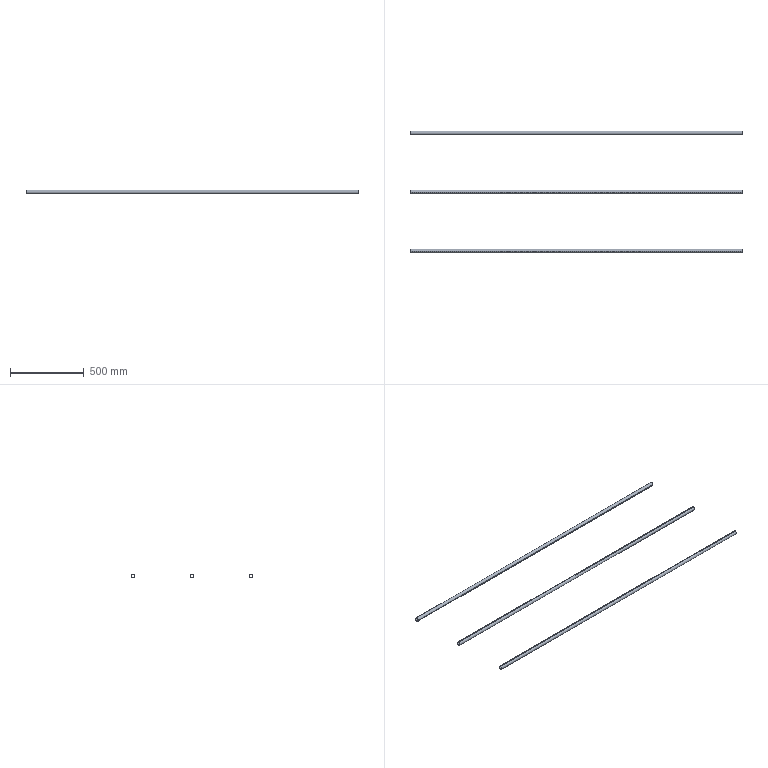Part | STEP file | 粉仓护栏栏杆6_Default<As Machined> | 3 solids | 18 faces | box 2250 x 825 x 25 mm | volume 747503 mm3 | cylinder 12 | plane 6 | commonest cylinder face diameters 22 x6 25 x6
STEP:
#1=CARTESIAN_POINT('',(0.,0.,0.));
#2=DIRECTION('',(0.,0.,1.));
#3=DIRECTION('',(1.,0.,0.));
#4=AXIS2_PLACEMENT_3D('',#1,#2,#3);
#5=CARTESIAN_POINT('',(-2250.,0.,12.5));
#6=VERTEX_POINT('',#5);
#7=CARTESIAN_POINT('',(-2250.,0.,-12.5));
#8=VERTEX_POINT('',#7);
#9=CARTESIAN_POINT('',(-2250.,0.,0.));
#10=DIRECTION('',(-1.,0.,0.));
#11=DIRECTION('',(0.,-1.,0.));
#12=AXIS2_PLACEMENT_3D('',#9,#10,#11);
#13=CIRCLE('',#12,12.5);
#14=CARTESIAN_POINT('',(-2250.,0.,0.));
#15=DIRECTION('',(1.,0.,0.));
#16=DIRECTION('',(0.,0.,-1.));
#17=AXIS2_PLACEMENT_3D('',#14,#15,#16);
#18=CYLINDRICAL_SURFACE('',#17,12.5);
#19=CARTESIAN_POINT('',(4.712,0.));
#20=DIRECTION('',(-1.,0.));
#21=VECTOR('',#20,1.);
#22=LINE('',#19,#21);
#23=(GEOMETRIC_REPRESENTATION_CONTEXT(2)PARAMETRIC_REPRESENTATION_CONTEXT()REPRESENTATION_CONTEXT('',''));
#24=DEFINITIONAL_REPRESENTATION('',(#22),#23);
#25=PCURVE('',#18,#24);
#26=CARTESIAN_POINT('',(-2250.,0.,0.));
#27=DIRECTION('',(-1.,0.,0.));
#28=DIRECTION('',(0.,-1.,0.));
#29=AXIS2_PLACEMENT_3D('',#26,#27,#28);
#30=PLANE('',#29);
#31=CARTESIAN_POINT('',(0.,0.));
#32=DIRECTION('',(1.,0.));
#33=AXIS2_PLACEMENT_2D('',#31,#32);
#34=CIRCLE('',#33,12.5);
#35=(GEOMETRIC_REPRESENTATION_CONTEXT(2)PARAMETRIC_REPRESENTATION_CONTEXT()REPRESENTATION_CONTEXT('',''));
#36=DEFINITIONAL_REPRESENTATION('',(#34),#35);
#37=PCURVE('',#30,#36);
#38=SURFACE_CURVE('',#13,(#25,#37),.PCURVE_S1.);
#39=EDGE_CURVE('',#6,#8,#38,.T.);
#40=ORIENTED_EDGE('',*,*,#39,.F.);
#41=CARTESIAN_POINT('',(0.,0.,12.5));
#42=VERTEX_POINT('',#41);
#43=CARTESIAN_POINT('',(-2250.,0.,12.5));
#44=DIRECTION('',(1.,0.,0.));
#45=VECTOR('',#44,1.);
#46=LINE('',#43,#45);
#47=CARTESIAN_POINT('',(3.142,0.));
#48=DIRECTION('',(0.,1.));
#49=VECTOR('',#48,1.);
#50=LINE('',#47,#49);
#51=(GEOMETRIC_REPRESENTATION_CONTEXT(2)PARAMETRIC_REPRESENTATION_CONTEXT()REPRESENTATION_CONTEXT('',''));
#52=DEFINITIONAL_REPRESENTATION('',(#50),#51);
#53=PCURVE('',#18,#52);
#54=CARTESIAN_POINT('',(-2250.,0.,0.));
#55=DIRECTION('',(1.,0.,0.));
#56=DIRECTION('',(0.,0.,-1.));
#57=AXIS2_PLACEMENT_3D('',#54,#55,#56);
#58=CYLINDRICAL_SURFACE('',#57,12.5);
#59=CARTESIAN_POINT('',(3.142,0.));
#60=DIRECTION('',(0.,1.));
#61=VECTOR('',#60,1.);
#62=LINE('',#59,#61);
#63=(GEOMETRIC_REPRESENTATION_CONTEXT(2)PARAMETRIC_REPRESENTATION_CONTEXT()REPRESENTATION_CONTEXT('',''));
#64=DEFINITIONAL_REPRESENTATION('',(#62),#63);
#65=PCURVE('',#58,#64);
#66=SURFACE_CURVE('',#46,(#53,#65),.PCURVE_S1.);
#67=EDGE_CURVE('',#6,#42,#66,.T.);
#68=ORIENTED_EDGE('',*,*,#67,.T.);
#69=CARTESIAN_POINT('',(0.,0.,-12.5));
#70=VERTEX_POINT('',#69);
#71=CARTESIAN_POINT('',(0.,0.,0.));
#72=DIRECTION('',(-1.,0.,0.));
#73=DIRECTION('',(0.,-1.,0.));
#74=AXIS2_PLACEMENT_3D('',#71,#72,#73);
#75=CIRCLE('',#74,12.5);
#76=CARTESIAN_POINT('',(4.712,2250.));
#77=DIRECTION('',(-1.,0.));
#78=VECTOR('',#77,1.);
#79=LINE('',#76,#78);
#80=(GEOMETRIC_REPRESENTATION_CONTEXT(2)PARAMETRIC_REPRESENTATION_CONTEXT()REPRESENTATION_CONTEXT('',''));
#81=DEFINITIONAL_REPRESENTATION('',(#79),#80);
#82=PCURVE('',#18,#81);
#83=CARTESIAN_POINT('',(0.,0.,0.));
#84=DIRECTION('',(-1.,0.,0.));
#85=DIRECTION('',(0.,-1.,0.));
#86=AXIS2_PLACEMENT_3D('',#83,#84,#85);
#87=PLANE('',#86);
#88=CARTESIAN_POINT('',(0.,0.));
#89=DIRECTION('',(1.,0.));
#90=AXIS2_PLACEMENT_2D('',#88,#89);
#91=CIRCLE('',#90,12.5);
#92=(GEOMETRIC_REPRESENTATION_CONTEXT(2)PARAMETRIC_REPRESENTATION_CONTEXT()REPRESENTATION_CONTEXT('',''));
#93=DEFINITIONAL_REPRESENTATION('',(#91),#92);
#94=PCURVE('',#87,#93);
#95=SURFACE_CURVE('',#75,(#82,#94),.PCURVE_S1.);
#96=EDGE_CURVE('',#42,#70,#95,.T.);
#97=ORIENTED_EDGE('',*,*,#96,.T.);
#98=CARTESIAN_POINT('',(-2250.,0.,-12.5));
#99=DIRECTION('',(1.,0.,0.));
#100=VECTOR('',#99,1.);
#101=LINE('',#98,#100);
#102=CARTESIAN_POINT('',(0.,0.));
#103=DIRECTION('',(0.,1.));
#104=VECTOR('',#103,1.);
#105=LINE('',#102,#104);
#106=(GEOMETRIC_REPRESENTATION_CONTEXT(2)PARAMETRIC_REPRESENTATION_CONTEXT()REPRESENTATION_CONTEXT('',''));
#107=DEFINITIONAL_REPRESENTATION('',(#105),#106);
#108=PCURVE('',#18,#107);
#109=CARTESIAN_POINT('',(6.283,0.));
#110=DIRECTION('',(0.,1.));
#111=VECTOR('',#110,1.);
#112=LINE('',#109,#111);
#113=(GEOMETRIC_REPRESENTATION_CONTEXT(2)PARAMETRIC_REPRESENTATION_CONTEXT()REPRESENTATION_CONTEXT('',''));
#114=DEFINITIONAL_REPRESENTATION('',(#112),#113);
#115=PCURVE('',#58,#114);
#116=SURFACE_CURVE('',#101,(#108,#115),.PCURVE_S1.);
#117=EDGE_CURVE('',#8,#70,#116,.T.);
#118=ORIENTED_EDGE('',*,*,#117,.F.);
#119=EDGE_LOOP('',(#40,#68,#97,#118));
#120=FACE_BOUND('',#119,.T.);
#121=ADVANCED_FACE('',(#120),#18,.T.);
#122=CARTESIAN_POINT('',(-2250.,0.,-11.));
#123=VERTEX_POINT('',#122);
#124=CARTESIAN_POINT('',(0.,0.,-11.));
#125=VERTEX_POINT('',#124);
#126=CARTESIAN_POINT('',(-2250.,0.,-11.));
#127=DIRECTION('',(1.,0.,0.));
#128=VECTOR('',#127,1.);
#129=LINE('',#126,#128);
#130=CARTESIAN_POINT('',(-2250.,0.,0.));
#131=DIRECTION('',(1.,0.,0.));
#132=DIRECTION('',(0.,0.,-1.));
#133=AXIS2_PLACEMENT_3D('',#130,#131,#132);
#134=CYLINDRICAL_SURFACE('',#133,11.);
#135=CARTESIAN_POINT('',(6.283,0.));
#136=DIRECTION('',(0.,1.));
#137=VECTOR('',#136,1.);
#138=LINE('',#135,#137);
#139=(GEOMETRIC_REPRESENTATION_CONTEXT(2)PARAMETRIC_REPRESENTATION_CONTEXT()REPRESENTATION_CONTEXT('',''));
#140=DEFINITIONAL_REPRESENTATION('',(#138),#139);
#141=PCURVE('',#134,#140);
#142=CARTESIAN_POINT('',(-2250.,0.,0.));
#143=DIRECTION('',(1.,0.,0.));
#144=DIRECTION('',(0.,0.,-1.));
#145=AXIS2_PLACEMENT_3D('',#142,#143,#144);
#146=CYLINDRICAL_SURFACE('',#145,11.);
#147=CARTESIAN_POINT('',(0.,0.));
#148=DIRECTION('',(0.,1.));
#149=VECTOR('',#148,1.);
#150=LINE('',#147,#149);
#151=(GEOMETRIC_REPRESENTATION_CONTEXT(2)PARAMETRIC_REPRESENTATION_CONTEXT()REPRESENTATION_CONTEXT('',''));
#152=DEFINITIONAL_REPRESENTATION('',(#150),#151);
#153=PCURVE('',#146,#152);
#154=SURFACE_CURVE('',#129,(#141,#153),.PCURVE_S1.);
#155=EDGE_CURVE('',#123,#125,#154,.T.);
#156=ORIENTED_EDGE('',*,*,#155,.T.);
#157=CARTESIAN_POINT('',(0.,0.,11.));
#158=VERTEX_POINT('',#157);
#159=CARTESIAN_POINT('',(0.,0.,0.));
#160=DIRECTION('',(-1.,0.,0.));
#161=DIRECTION('',(0.,-1.,0.));
#162=AXIS2_PLACEMENT_3D('',#159,#160,#161);
#163=CIRCLE('',#162,11.);
#164=CARTESIAN_POINT('',(10.996,2250.));
#165=DIRECTION('',(-1.,0.));
#166=VECTOR('',#165,1.);
#167=LINE('',#164,#166);
#168=(GEOMETRIC_REPRESENTATION_CONTEXT(2)PARAMETRIC_REPRESENTATION_CONTEXT()REPRESENTATION_CONTEXT('',''));
#169=DEFINITIONAL_REPRESENTATION('',(#167),#168);
#170=PCURVE('',#134,#169);
#171=CARTESIAN_POINT('',(0.,0.));
#172=DIRECTION('',(1.,0.));
#173=AXIS2_PLACEMENT_2D('',#171,#172);
#174=CIRCLE('',#173,11.);
#175=(GEOMETRIC_REPRESENTATION_CONTEXT(2)PARAMETRIC_REPRESENTATION_CONTEXT()REPRESENTATION_CONTEXT('',''));
#176=DEFINITIONAL_REPRESENTATION('',(#174),#175);
#177=PCURVE('',#87,#176);
#178=SURFACE_CURVE('',#163,(#170,#177),.PCURVE_S1.);
#179=EDGE_CURVE('',#125,#158,#178,.T.);
#180=ORIENTED_EDGE('',*,*,#179,.T.);
#181=CARTESIAN_POINT('',(-2250.,0.,11.));
#182=VERTEX_POINT('',#181);
#183=CARTESIAN_POINT('',(-2250.,0.,11.));
#184=DIRECTION('',(1.,0.,0.));
#185=VECTOR('',#184,1.);
#186=LINE('',#183,#185);
#187=CARTESIAN_POINT('',(3.142,0.));
#188=DIRECTION('',(0.,1.));
#189=VECTOR('',#188,1.);
#190=LINE('',#187,#189);
#191=(GEOMETRIC_REPRESENTATION_CONTEXT(2)PARAMETRIC_REPRESENTATION_CONTEXT()REPRESENTATION_CONTEXT('',''));
#192=DEFINITIONAL_REPRESENTATION('',(#190),#191);
#193=PCURVE('',#134,#192);
#194=CARTESIAN_POINT('',(3.142,0.));
#195=DIRECTION('',(0.,1.));
#196=VECTOR('',#195,1.);
#197=LINE('',#194,#196);
#198=(GEOMETRIC_REPRESENTATION_CONTEXT(2)PARAMETRIC_REPRESENTATION_CONTEXT()REPRESENTATION_CONTEXT('',''));
#199=DEFINITIONAL_REPRESENTATION('',(#197),#198);
#200=PCURVE('',#146,#199);
#201=SURFACE_CURVE('',#186,(#193,#200),.PCURVE_S1.);
#202=EDGE_CURVE('',#182,#158,#201,.T.);
#203=ORIENTED_EDGE('',*,*,#202,.F.);
#204=CARTESIAN_POINT('',(-2250.,0.,0.));
#205=DIRECTION('',(-1.,0.,0.));
#206=DIRECTION('',(0.,-1.,0.));
#207=AXIS2_PLACEMENT_3D('',#204,#205,#206);
#208=CIRCLE('',#207,11.);
#209=CARTESIAN_POINT('',(10.996,0.));
#210=DIRECTION('',(-1.,0.));
#211=VECTOR('',#210,1.);
#212=LINE('',#209,#211);
#213=(GEOMETRIC_REPRESENTATION_CONTEXT(2)PARAMETRIC_REPRESENTATION_CONTEXT()REPRESENTATION_CONTEXT('',''));
#214=DEFINITIONAL_REPRESENTATION('',(#212),#213);
#215=PCURVE('',#134,#214);
#216=CARTESIAN_POINT('',(0.,0.));
#217=DIRECTION('',(1.,0.));
#218=AXIS2_PLACEMENT_2D('',#216,#217);
#219=CIRCLE('',#218,11.);
#220=(GEOMETRIC_REPRESENTATION_CONTEXT(2)PARAMETRIC_REPRESENTATION_CONTEXT()REPRESENTATION_CONTEXT('',''));
#221=DEFINITIONAL_REPRESENTATION('',(#219),#220);
#222=PCURVE('',#30,#221);
#223=SURFACE_CURVE('',#208,(#215,#222),.PCURVE_S1.);
#224=EDGE_CURVE('',#123,#182,#223,.T.);
#225=ORIENTED_EDGE('',*,*,#224,.F.);
#226=EDGE_LOOP('',(#156,#180,#203,#225));
#227=FACE_BOUND('',#226,.F.);
#228=ADVANCED_FACE('',(#227),#134,.F.);
#229=CARTESIAN_POINT('',(0.,0.,0.));
#230=DIRECTION('',(-1.,0.,0.));
#231=DIRECTION('',(0.,-1.,0.));
#232=AXIS2_PLACEMENT_3D('',#229,#230,#231);
#233=CIRCLE('',#232,11.);
#234=CARTESIAN_POINT('',(4.712,2250.));
#235=DIRECTION('',(-1.,0.));
#236=VECTOR('',#235,1.);
#237=LINE('',#234,#236);
#238=(GEOMETRIC_REPRESENTATION_CONTEXT(2)PARAMETRIC_REPRESENTATION_CONTEXT()REPRESENTATION_CONTEXT('',''));
#239=DEFINITIONAL_REPRESENTATION('',(#237),#238);
#240=PCURVE('',#146,#239);
#241=CARTESIAN_POINT('',(0.,0.));
#242=DIRECTION('',(1.,0.));
#243=AXIS2_PLACEMENT_2D('',#241,#242);
#244=CIRCLE('',#243,11.);
#245=(GEOMETRIC_REPRESENTATION_CONTEXT(2)PARAMETRIC_REPRESENTATION_CONTEXT()REPRESENTATION_CONTEXT('',''));
#246=DEFINITIONAL_REPRESENTATION('',(#244),#245);
#247=PCURVE('',#87,#246);
#248=SURFACE_CURVE('',#233,(#240,#247),.PCURVE_S1.);
#249=EDGE_CURVE('',#158,#125,#248,.T.);
#250=ORIENTED_EDGE('',*,*,#249,.T.);
#251=ORIENTED_EDGE('',*,*,#155,.F.);
#252=CARTESIAN_POINT('',(-2250.,0.,0.));
#253=DIRECTION('',(-1.,0.,0.));
#254=DIRECTION('',(0.,-1.,0.));
#255=AXIS2_PLACEMENT_3D('',#252,#253,#254);
#256=CIRCLE('',#255,11.);
#257=CARTESIAN_POINT('',(4.712,0.));
#258=DIRECTION('',(-1.,0.));
#259=VECTOR('',#258,1.);
#260=LINE('',#257,#259);
#261=(GEOMETRIC_REPRESENTATION_CONTEXT(2)PARAMETRIC_REPRESENTATION_CONTEXT()REPRESENTATION_CONTEXT('',''));
#262=DEFINITIONAL_REPRESENTATION('',(#260),#261);
#263=PCURVE('',#146,#262);
#264=CARTESIAN_POINT('',(0.,0.));
#265=DIRECTION('',(1.,0.));
#266=AXIS2_PLACEMENT_2D('',#264,#265);
#267=CIRCLE('',#266,11.);
#268=(GEOMETRIC_REPRESENTATION_CONTEXT(2)PARAMETRIC_REPRESENTATION_CONTEXT()REPRESENTATION_CONTEXT('',''));
#269=DEFINITIONAL_REPRESENTATION('',(#267),#268);
#270=PCURVE('',#30,#269);
#271=SURFACE_CURVE('',#256,(#263,#270),.PCURVE_S1.);
#272=EDGE_CURVE('',#182,#123,#271,.T.);
#273=ORIENTED_EDGE('',*,*,#272,.F.);
#274=ORIENTED_EDGE('',*,*,#202,.T.);
#275=EDGE_LOOP('',(#250,#251,#273,#274));
#276=FACE_BOUND('',#275,.F.);
#277=ADVANCED_FACE('',(#276),#146,.F.);
#278=ORIENTED_EDGE('',*,*,#67,.F.);
#279=CARTESIAN_POINT('',(-2250.,0.,0.));
#280=DIRECTION('',(-1.,0.,0.));
#281=DIRECTION('',(0.,-1.,0.));
#282=AXIS2_PLACEMENT_3D('',#279,#280,#281);
#283=CIRCLE('',#282,12.5);
#284=CARTESIAN_POINT('',(10.996,0.));
#285=DIRECTION('',(-1.,0.));
#286=VECTOR('',#285,1.);
#287=LINE('',#284,#286);
#288=(GEOMETRIC_REPRESENTATION_CONTEXT(2)PARAMETRIC_REPRESENTATION_CONTEXT()REPRESENTATION_CONTEXT('',''));
#289=DEFINITIONAL_REPRESENTATION('',(#287),#288);
#290=PCURVE('',#58,#289);
#291=CARTESIAN_POINT('',(0.,0.));
#292=DIRECTION('',(1.,0.));
#293=AXIS2_PLACEMENT_2D('',#291,#292);
#294=CIRCLE('',#293,12.5);
#295=(GEOMETRIC_REPRESENTATION_CONTEXT(2)PARAMETRIC_REPRESENTATION_CONTEXT()REPRESENTATION_CONTEXT('',''));
#296=DEFINITIONAL_REPRESENTATION('',(#294),#295);
#297=PCURVE('',#30,#296);
#298=SURFACE_CURVE('',#283,(#290,#297),.PCURVE_S1.);
#299=EDGE_CURVE('',#8,#6,#298,.T.);
#300=ORIENTED_EDGE('',*,*,#299,.F.);
#301=ORIENTED_EDGE('',*,*,#117,.T.);
#302=CARTESIAN_POINT('',(0.,0.,0.));
#303=DIRECTION('',(-1.,0.,0.));
#304=DIRECTION('',(0.,-1.,0.));
#305=AXIS2_PLACEMENT_3D('',#302,#303,#304);
#306=CIRCLE('',#305,12.5);
#307=CARTESIAN_POINT('',(10.996,2250.));
#308=DIRECTION('',(-1.,0.));
#309=VECTOR('',#308,1.);
#310=LINE('',#307,#309);
#311=(GEOMETRIC_REPRESENTATION_CONTEXT(2)PARAMETRIC_REPRESENTATION_CONTEXT()REPRESENTATION_CONTEXT('',''));
#312=DEFINITIONAL_REPRESENTATION('',(#310),#311);
#313=PCURVE('',#58,#312);
#314=CARTESIAN_POINT('',(0.,0.));
#315=DIRECTION('',(1.,0.));
#316=AXIS2_PLACEMENT_2D('',#314,#315);
#317=CIRCLE('',#316,12.5);
#318=(GEOMETRIC_REPRESENTATION_CONTEXT(2)PARAMETRIC_REPRESENTATION_CONTEXT()REPRESENTATION_CONTEXT('',''));
#319=DEFINITIONAL_REPRESENTATION('',(#317),#318);
#320=PCURVE('',#87,#319);
#321=SURFACE_CURVE('',#306,(#313,#320),.PCURVE_S1.);
#322=EDGE_CURVE('',#70,#42,#321,.T.);
#323=ORIENTED_EDGE('',*,*,#322,.T.);
#324=EDGE_LOOP('',(#278,#300,#301,#323));
#325=FACE_BOUND('',#324,.T.);
#326=ADVANCED_FACE('',(#325),#58,.T.);
#327=ORIENTED_EDGE('',*,*,#224,.F.);
#328=ORIENTED_EDGE('',*,*,#272,.F.);
#329=EDGE_LOOP('',(#327,#328));
#330=FACE_BOUND('',#329,.T.);
#331=ORIENTED_EDGE('',*,*,#299,.T.);
#332=ORIENTED_EDGE('',*,*,#39,.T.);
#333=EDGE_LOOP('',(#331,#332));
#334=FACE_BOUND('',#333,.T.);
#335=ADVANCED_FACE('',(#330,#334),#30,.T.);
#336=ORIENTED_EDGE('',*,*,#179,.T.);
#337=ORIENTED_EDGE('',*,*,#249,.T.);
#338=EDGE_LOOP('',(#336,#337));
#339=FACE_BOUND('',#338,.T.);
#340=ORIENTED_EDGE('',*,*,#322,.F.);
#341=ORIENTED_EDGE('',*,*,#96,.F.);
#342=EDGE_LOOP('',(#340,#341));
#343=FACE_BOUND('',#342,.T.);
#344=ADVANCED_FACE('',(#339,#343),#87,.F.);
#345=CLOSED_SHELL('',(#121,#228,#277,#326,#335,#344));
#346=MANIFOLD_SOLID_BREP('',#345);
#347=CARTESIAN_POINT('',(-2250.,787.5,0.));
#348=VERTEX_POINT('',#347);
#349=CARTESIAN_POINT('',(-2250.,812.5,0.));
#350=VERTEX_POINT('',#349);
#351=CARTESIAN_POINT('',(-2250.,800.,0.));
#352=DIRECTION('',(-1.,0.,0.));
#353=DIRECTION('',(0.,-1.,0.));
#354=AXIS2_PLACEMENT_3D('',#351,#352,#353);
#355=CIRCLE('',#354,12.5);
#356=CARTESIAN_POINT('',(-2250.,800.,0.));
#357=DIRECTION('',(1.,0.,0.));
#358=DIRECTION('',(0.,1.,0.));
#359=AXIS2_PLACEMENT_3D('',#356,#357,#358);
#360=CYLINDRICAL_SURFACE('',#359,12.5);
#361=CARTESIAN_POINT('',(3.142,0.));
#362=DIRECTION('',(-1.,0.));
#363=VECTOR('',#362,1.);
#364=LINE('',#361,#363);
#365=(GEOMETRIC_REPRESENTATION_CONTEXT(2)PARAMETRIC_REPRESENTATION_CONTEXT()REPRESENTATION_CONTEXT('',''));
#366=DEFINITIONAL_REPRESENTATION('',(#364),#365);
#367=PCURVE('',#360,#366);
#368=CARTESIAN_POINT('',(-2250.,800.,0.));
#369=DIRECTION('',(-1.,0.,0.));
#370=DIRECTION('',(0.,-1.,0.));
#371=AXIS2_PLACEMENT_3D('',#368,#369,#370);
#372=PLANE('',#371);
#373=CARTESIAN_POINT('',(0.,0.));
#374=DIRECTION('',(1.,0.));
#375=AXIS2_PLACEMENT_2D('',#373,#374);
#376=CIRCLE('',#375,12.5);
#377=(GEOMETRIC_REPRESENTATION_CONTEXT(2)PARAMETRIC_REPRESENTATION_CONTEXT()REPRESENTATION_CONTEXT('',''));
#378=DEFINITIONAL_REPRESENTATION('',(#376),#377);
#379=PCURVE('',#372,#378);
#380=SURFACE_CURVE('',#355,(#367,#379),.PCURVE_S1.);
#381=EDGE_CURVE('',#348,#350,#380,.T.);
#382=ORIENTED_EDGE('',*,*,#381,.F.);
#383=CARTESIAN_POINT('',(0.,787.5,0.));
#384=VERTEX_POINT('',#383);
#385=CARTESIAN_POINT('',(-2250.,787.5,0.));
#386=DIRECTION('',(1.,0.,0.));
#387=VECTOR('',#386,1.);
#388=LINE('',#385,#387);
#389=CARTESIAN_POINT('',(3.142,0.));
#390=DIRECTION('',(0.,1.));
#391=VECTOR('',#390,1.);
#392=LINE('',#389,#391);
#393=(GEOMETRIC_REPRESENTATION_CONTEXT(2)PARAMETRIC_REPRESENTATION_CONTEXT()REPRESENTATION_CONTEXT('',''));
#394=DEFINITIONAL_REPRESENTATION('',(#392),#393);
#395=PCURVE('',#360,#394);
#396=CARTESIAN_POINT('',(-2250.,800.,0.));
#397=DIRECTION('',(1.,0.,0.));
#398=DIRECTION('',(0.,1.,0.));
#399=AXIS2_PLACEMENT_3D('',#396,#397,#398);
#400=CYLINDRICAL_SURFACE('',#399,12.5);
#401=CARTESIAN_POINT('',(3.142,0.));
#402=DIRECTION('',(0.,1.));
#403=VECTOR('',#402,1.);
#404=LINE('',#401,#403);
#405=(GEOMETRIC_REPRESENTATION_CONTEXT(2)PARAMETRIC_REPRESENTATION_CONTEXT()REPRESENTATION_CONTEXT('',''));
#406=DEFINITIONAL_REPRESENTATION('',(#404),#405);
#407=PCURVE('',#400,#406);
#408=SURFACE_CURVE('',#388,(#395,#407),.PCURVE_S1.);
#409=EDGE_CURVE('',#348,#384,#408,.T.);
#410=ORIENTED_EDGE('',*,*,#409,.T.);
#411=CARTESIAN_POINT('',(0.,812.5,0.));
#412=VERTEX_POINT('',#411);
#413=CARTESIAN_POINT('',(0.,800.,0.));
#414=DIRECTION('',(-1.,0.,0.));
#415=DIRECTION('',(0.,-1.,0.));
#416=AXIS2_PLACEMENT_3D('',#413,#414,#415);
#417=CIRCLE('',#416,12.5);
#418=CARTESIAN_POINT('',(3.142,2250.));
#419=DIRECTION('',(-1.,0.));
#420=VECTOR('',#419,1.);
#421=LINE('',#418,#420);
#422=(GEOMETRIC_REPRESENTATION_CONTEXT(2)PARAMETRIC_REPRESENTATION_CONTEXT()REPRESENTATION_CONTEXT('',''));
#423=DEFINITIONAL_REPRESENTATION('',(#421),#422);
#424=PCURVE('',#360,#423);
#425=CARTESIAN_POINT('',(0.,800.,0.));
#426=DIRECTION('',(-1.,0.,0.));
#427=DIRECTION('',(0.,-1.,0.));
#428=AXIS2_PLACEMENT_3D('',#425,#426,#427);
#429=PLANE('',#428);
#430=CARTESIAN_POINT('',(0.,0.));
#431=DIRECTION('',(1.,0.));
#432=AXIS2_PLACEMENT_2D('',#430,#431);
#433=CIRCLE('',#432,12.5);
#434=(GEOMETRIC_REPRESENTATION_CONTEXT(2)PARAMETRIC_REPRESENTATION_CONTEXT()REPRESENTATION_CONTEXT('',''));
#435=DEFINITIONAL_REPRESENTATION('',(#433),#434);
#436=PCURVE('',#429,#435);
#437=SURFACE_CURVE('',#417,(#424,#436),.PCURVE_S1.);
#438=EDGE_CURVE('',#384,#412,#437,.T.);
#439=ORIENTED_EDGE('',*,*,#438,.T.);
#440=CARTESIAN_POINT('',(-2250.,812.5,0.));
#441=DIRECTION('',(1.,0.,0.));
#442=VECTOR('',#441,1.);
#443=LINE('',#440,#442);
#444=CARTESIAN_POINT('',(0.,0.));
#445=DIRECTION('',(0.,1.));
#446=VECTOR('',#445,1.);
#447=LINE('',#444,#446);
#448=(GEOMETRIC_REPRESENTATION_CONTEXT(2)PARAMETRIC_REPRESENTATION_CONTEXT()REPRESENTATION_CONTEXT('',''));
#449=DEFINITIONAL_REPRESENTATION('',(#447),#448);
#450=PCURVE('',#360,#449);
#451=CARTESIAN_POINT('',(6.283,0.));
#452=DIRECTION('',(0.,1.));
#453=VECTOR('',#452,1.);
#454=LINE('',#451,#453);
#455=(GEOMETRIC_REPRESENTATION_CONTEXT(2)PARAMETRIC_REPRESENTATION_CONTEXT()REPRESENTATION_CONTEXT('',''));
#456=DEFINITIONAL_REPRESENTATION('',(#454),#455);
#457=PCURVE('',#400,#456);
#458=SURFACE_CURVE('',#443,(#450,#457),.PCURVE_S1.);
#459=EDGE_CURVE('',#350,#412,#458,.T.);
#460=ORIENTED_EDGE('',*,*,#459,.F.);
#461=EDGE_LOOP('',(#382,#410,#439,#460));
#462=FACE_BOUND('',#461,.T.);
#463=ADVANCED_FACE('',(#462),#360,.T.);
#464=CARTESIAN_POINT('',(-2250.,811.,0.));
#465=VERTEX_POINT('',#464);
#466=CARTESIAN_POINT('',(0.,811.,0.));
#467=VERTEX_POINT('',#466);
#468=CARTESIAN_POINT('',(-2250.,811.,0.));
#469=DIRECTION('',(1.,0.,0.));
#470=VECTOR('',#469,1.);
#471=LINE('',#468,#470);
#472=CARTESIAN_POINT('',(-2250.,800.,0.));
#473=DIRECTION('',(1.,0.,0.));
#474=DIRECTION('',(0.,1.,0.));
#475=AXIS2_PLACEMENT_3D('',#472,#473,#474);
#476=CYLINDRICAL_SURFACE('',#475,11.);
#477=CARTESIAN_POINT('',(6.283,0.));
#478=DIRECTION('',(0.,1.));
#479=VECTOR('',#478,1.);
#480=LINE('',#477,#479);
#481=(GEOMETRIC_REPRESENTATION_CONTEXT(2)PARAMETRIC_REPRESENTATION_CONTEXT()REPRESENTATION_CONTEXT('',''));
#482=DEFINITIONAL_REPRESENTATION('',(#480),#481);
#483=PCURVE('',#476,#482);
#484=CARTESIAN_POINT('',(-2250.,800.,0.));
#485=DIRECTION('',(1.,0.,0.));
#486=DIRECTION('',(0.,1.,0.));
#487=AXIS2_PLACEMENT_3D('',#484,#485,#486);
#488=CYLINDRICAL_SURFACE('',#487,11.);
#489=CARTESIAN_POINT('',(0.,0.));
#490=DIRECTION('',(0.,1.));
#491=VECTOR('',#490,1.);
#492=LINE('',#489,#491);
#493=(GEOMETRIC_REPRESENTATION_CONTEXT(2)PARAMETRIC_REPRESENTATION_CONTEXT()REPRESENTATION_CONTEXT('',''));
#494=DEFINITIONAL_REPRESENTATION('',(#492),#493);
#495=PCURVE('',#488,#494);
#496=SURFACE_CURVE('',#471,(#483,#495),.PCURVE_S1.);
#497=EDGE_CURVE('',#465,#467,#496,.T.);
#498=ORIENTED_EDGE('',*,*,#497,.T.);
#499=CARTESIAN_POINT('',(0.,789.,0.));
#500=VERTEX_POINT('',#499);
#501=CARTESIAN_POINT('',(0.,800.,0.));
#502=DIRECTION('',(-1.,0.,0.));
#503=DIRECTION('',(0.,-1.,0.));
#504=AXIS2_PLACEMENT_3D('',#501,#502,#503);
#505=CIRCLE('',#504,11.);
#506=CARTESIAN_POINT('',(9.425,2250.));
#507=DIRECTION('',(-1.,0.));
#508=VECTOR('',#507,1.);
#509=LINE('',#506,#508);
#510=(GEOMETRIC_REPRESENTATION_CONTEXT(2)PARAMETRIC_REPRESENTATION_CONTEXT()REPRESENTATION_CONTEXT('',''));
#511=DEFINITIONAL_REPRESENTATION('',(#509),#510);
#512=PCURVE('',#476,#511);
#513=CARTESIAN_POINT('',(0.,0.));
#514=DIRECTION('',(1.,0.));
#515=AXIS2_PLACEMENT_2D('',#513,#514);
#516=CIRCLE('',#515,11.);
#517=(GEOMETRIC_REPRESENTATION_CONTEXT(2)PARAMETRIC_REPRESENTATION_CONTEXT()REPRESENTATION_CONTEXT('',''));
#518=DEFINITIONAL_REPRESENTATION('',(#516),#517);
#519=PCURVE('',#429,#518);
#520=SURFACE_CURVE('',#505,(#512,#519),.PCURVE_S1.);
#521=EDGE_CURVE('',#467,#500,#520,.T.);
#522=ORIENTED_EDGE('',*,*,#521,.T.);
#523=CARTESIAN_POINT('',(-2250.,789.,0.));
#524=VERTEX_POINT('',#523);
#525=CARTESIAN_POINT('',(-2250.,789.,0.));
#526=DIRECTION('',(1.,0.,0.));
#527=VECTOR('',#526,1.);
#528=LINE('',#525,#527);
#529=CARTESIAN_POINT('',(3.142,0.));
#530=DIRECTION('',(0.,1.));
#531=VECTOR('',#530,1.);
#532=LINE('',#529,#531);
#533=(GEOMETRIC_REPRESENTATION_CONTEXT(2)PARAMETRIC_REPRESENTATION_CONTEXT()REPRESENTATION_CONTEXT('',''));
#534=DEFINITIONAL_REPRESENTATION('',(#532),#533);
#535=PCURVE('',#476,#534);
#536=CARTESIAN_POINT('',(3.142,0.));
#537=DIRECTION('',(0.,1.));
#538=VECTOR('',#537,1.);
#539=LINE('',#536,#538);
#540=(GEOMETRIC_REPRESENTATION_CONTEXT(2)PARAMETRIC_REPRESENTATION_CONTEXT()REPRESENTATION_CONTEXT('',''));
#541=DEFINITIONAL_REPRESENTATION('',(#539),#540);
#542=PCURVE('',#488,#541);
#543=SURFACE_CURVE('',#528,(#535,#542),.PCURVE_S1.);
#544=EDGE_CURVE('',#524,#500,#543,.T.);
#545=ORIENTED_EDGE('',*,*,#544,.F.);
#546=CARTESIAN_POINT('',(-2250.,800.,0.));
#547=DIRECTION('',(-1.,0.,0.));
#548=DIRECTION('',(0.,-1.,0.));
#549=AXIS2_PLACEMENT_3D('',#546,#547,#548);
#550=CIRCLE('',#549,11.);
#551=CARTESIAN_POINT('',(9.425,0.));
#552=DIRECTION('',(-1.,0.));
#553=VECTOR('',#552,1.);
#554=LINE('',#551,#553);
#555=(GEOMETRIC_REPRESENTATION_CONTEXT(2)PARAMETRIC_REPRESENTATION_CONTEXT()REPRESENTATION_CONTEXT('',''));
#556=DEFINITIONAL_REPRESENTATION('',(#554),#555);
#557=PCURVE('',#476,#556);
#558=CARTESIAN_POINT('',(0.,0.));
#559=DIRECTION('',(1.,0.));
#560=AXIS2_PLACEMENT_2D('',#558,#559);
#561=CIRCLE('',#560,11.);
#562=(GEOMETRIC_REPRESENTATION_CONTEXT(2)PARAMETRIC_REPRESENTATION_CONTEXT()REPRESENTATION_CONTEXT('',''));
#563=DEFINITIONAL_REPRESENTATION('',(#561),#562);
#564=PCURVE('',#372,#563);
#565=SURFACE_CURVE('',#550,(#557,#564),.PCURVE_S1.);
#566=EDGE_CURVE('',#465,#524,#565,.T.);
#567=ORIENTED_EDGE('',*,*,#566,.F.);
#568=EDGE_LOOP('',(#498,#522,#545,#567));
#569=FACE_BOUND('',#568,.F.);
#570=ADVANCED_FACE('',(#569),#476,.F.);
#571=CARTESIAN_POINT('',(0.,800.,0.));
#572=DIRECTION('',(-1.,0.,0.));
#573=DIRECTION('',(0.,-1.,0.));
#574=AXIS2_PLACEMENT_3D('',#571,#572,#573);
#575=CIRCLE('',#574,11.);
#576=CARTESIAN_POINT('',(3.142,2250.));
#577=DIRECTION('',(-1.,0.));
#578=VECTOR('',#577,1.);
#579=LINE('',#576,#578);
#580=(GEOMETRIC_REPRESENTATION_CONTEXT(2)PARAMETRIC_REPRESENTATION_CONTEXT()REPRESENTATION_CONTEXT('',''));
#581=DEFINITIONAL_REPRESENTATION('',(#579),#580);
#582=PCURVE('',#488,#581);
#583=CARTESIAN_POINT('',(0.,0.));
#584=DIRECTION('',(1.,0.));
#585=AXIS2_PLACEMENT_2D('',#583,#584);
#586=CIRCLE('',#585,11.);
#587=(GEOMETRIC_REPRESENTATION_CONTEXT(2)PARAMETRIC_REPRESENTATION_CONTEXT()REPRESENTATION_CONTEXT('',''));
#588=DEFINITIONAL_REPRESENTATION('',(#586),#587);
#589=PCURVE('',#429,#588);
#590=SURFACE_CURVE('',#575,(#582,#589),.PCURVE_S1.);
#591=EDGE_CURVE('',#500,#467,#590,.T.);
#592=ORIENTED_EDGE('',*,*,#591,.T.);
#593=ORIENTED_EDGE('',*,*,#497,.F.);
#594=CARTESIAN_POINT('',(-2250.,800.,0.));
#595=DIRECTION('',(-1.,0.,0.));
#596=DIRECTION('',(0.,-1.,0.));
#597=AXIS2_PLACEMENT_3D('',#594,#595,#596);
#598=CIRCLE('',#597,11.);
#599=CARTESIAN_POINT('',(3.142,0.));
#600=DIRECTION('',(-1.,0.));
#601=VECTOR('',#600,1.);
#602=LINE('',#599,#601);
#603=(GEOMETRIC_REPRESENTATION_CONTEXT(2)PARAMETRIC_REPRESENTATION_CONTEXT()REPRESENTATION_CONTEXT('',''));
#604=DEFINITIONAL_REPRESENTATION('',(#602),#603);
#605=PCURVE('',#488,#604);
#606=CARTESIAN_POINT('',(0.,0.));
#607=DIRECTION('',(1.,0.));
#608=AXIS2_PLACEMENT_2D('',#606,#607);
#609=CIRCLE('',#608,11.);
#610=(GEOMETRIC_REPRESENTATION_CONTEXT(2)PARAMETRIC_REPRESENTATION_CONTEXT()REPRESENTATION_CONTEXT('',''));
#611=DEFINITIONAL_REPRESENTATION('',(#609),#610);
#612=PCURVE('',#372,#611);
#613=SURFACE_CURVE('',#598,(#605,#612),.PCURVE_S1.);
#614=EDGE_CURVE('',#524,#465,#613,.T.);
#615=ORIENTED_EDGE('',*,*,#614,.F.);
#616=ORIENTED_EDGE('',*,*,#544,.T.);
#617=EDGE_LOOP('',(#592,#593,#615,#616));
#618=FACE_BOUND('',#617,.F.);
#619=ADVANCED_FACE('',(#618),#488,.F.);
#620=ORIENTED_EDGE('',*,*,#409,.F.);
#621=CARTESIAN_POINT('',(-2250.,800.,0.));
#622=DIRECTION('',(-1.,0.,0.));
#623=DIRECTION('',(0.,-1.,0.));
#624=AXIS2_PLACEMENT_3D('',#621,#622,#623);
#625=CIRCLE('',#624,12.5);
#626=CARTESIAN_POINT('',(9.425,0.));
#627=DIRECTION('',(-1.,0.));
#628=VECTOR('',#627,1.);
#629=LINE('',#626,#628);
#630=(GEOMETRIC_REPRESENTATION_CONTEXT(2)PARAMETRIC_REPRESENTATION_CONTEXT()REPRESENTATION_CONTEXT('',''));
#631=DEFINITIONAL_REPRESENTATION('',(#629),#630);
#632=PCURVE('',#400,#631);
#633=CARTESIAN_POINT('',(0.,0.));
#634=DIRECTION('',(1.,0.));
#635=AXIS2_PLACEMENT_2D('',#633,#634);
#636=CIRCLE('',#635,12.5);
#637=(GEOMETRIC_REPRESENTATION_CONTEXT(2)PARAMETRIC_REPRESENTATION_CONTEXT()REPRESENTATION_CONTEXT('',''));
#638=DEFINITIONAL_REPRESENTATION('',(#636),#637);
#639=PCURVE('',#372,#638);
#640=SURFACE_CURVE('',#625,(#632,#639),.PCURVE_S1.);
#641=EDGE_CURVE('',#350,#348,#640,.T.);
#642=ORIENTED_EDGE('',*,*,#641,.F.);
#643=ORIENTED_EDGE('',*,*,#459,.T.);
#644=CARTESIAN_POINT('',(0.,800.,0.));
#645=DIRECTION('',(-1.,0.,0.));
#646=DIRECTION('',(0.,-1.,0.));
#647=AXIS2_PLACEMENT_3D('',#644,#645,#646);
#648=CIRCLE('',#647,12.5);
#649=CARTESIAN_POINT('',(9.425,2250.));
#650=DIRECTION('',(-1.,0.));
#651=VECTOR('',#650,1.);
#652=LINE('',#649,#651);
#653=(GEOMETRIC_REPRESENTATION_CONTEXT(2)PARAMETRIC_REPRESENTATION_CONTEXT()REPRESENTATION_CONTEXT('',''));
#654=DEFINITIONAL_REPRESENTATION('',(#652),#653);
#655=PCURVE('',#400,#654);
#656=CARTESIAN_POINT('',(0.,0.));
#657=DIRECTION('',(1.,0.));
#658=AXIS2_PLACEMENT_2D('',#656,#657);
#659=CIRCLE('',#658,12.5);
#660=(GEOMETRIC_REPRESENTATION_CONTEXT(2)PARAMETRIC_REPRESENTATION_CONTEXT()REPRESENTATION_CONTEXT('',''));
#661=DEFINITIONAL_REPRESENTATION('',(#659),#660);
#662=PCURVE('',#429,#661);
#663=SURFACE_CURVE('',#648,(#655,#662),.PCURVE_S1.);
#664=EDGE_CURVE('',#412,#384,#663,.T.);
#665=ORIENTED_EDGE('',*,*,#664,.T.);
#666=EDGE_LOOP('',(#620,#642,#643,#665));
#667=FACE_BOUND('',#666,.T.);
#668=ADVANCED_FACE('',(#667),#400,.T.);
#669=ORIENTED_EDGE('',*,*,#566,.F.);
#670=ORIENTED_EDGE('',*,*,#614,.F.);
#671=EDGE_LOOP('',(#669,#670));
#672=FACE_BOUND('',#671,.T.);
#673=ORIENTED_EDGE('',*,*,#641,.T.);
#674=ORIENTED_EDGE('',*,*,#381,.T.);
#675=EDGE_LOOP('',(#673,#674));
#676=FACE_BOUND('',#675,.T.);
#677=ADVANCED_FACE('',(#672,#676),#372,.T.);
#678=ORIENTED_EDGE('',*,*,#521,.T.);
#679=ORIENTED_EDGE('',*,*,#591,.T.);
#680=EDGE_LOOP('',(#678,#679));
#681=FACE_BOUND('',#680,.T.);
#682=ORIENTED_EDGE('',*,*,#664,.F.);
#683=ORIENTED_EDGE('',*,*,#438,.F.);
#684=EDGE_LOOP('',(#682,#683));
#685=FACE_BOUND('',#684,.T.);
#686=ADVANCED_FACE('',(#681,#685),#429,.F.);
#687=CLOSED_SHELL('',(#463,#570,#619,#668,#677,#686));
#688=MANIFOLD_SOLID_BREP('',#687);
#689=CARTESIAN_POINT('',(0.,400.,-12.5));
#690=VERTEX_POINT('',#689);
#691=CARTESIAN_POINT('',(0.,400.,12.5));
#692=VERTEX_POINT('',#691);
#693=CARTESIAN_POINT('',(0.,400.,0.));
#694=DIRECTION('',(1.,0.,0.));
#695=DIRECTION('',(0.,1.,0.));
#696=AXIS2_PLACEMENT_3D('',#693,#694,#695);
#697=CIRCLE('',#696,12.5);
#698=CARTESIAN_POINT('',(0.,400.,0.));
#699=DIRECTION('',(-1.,0.,0.));
#700=DIRECTION('',(0.,0.,1.));
#701=AXIS2_PLACEMENT_3D('',#698,#699,#700);
#702=CYLINDRICAL_SURFACE('',#701,12.5);
#703=CARTESIAN_POINT('',(7.854,0.));
#704=DIRECTION('',(-1.,0.));
#705=VECTOR('',#704,1.);
#706=LINE('',#703,#705);
#707=(GEOMETRIC_REPRESENTATION_CONTEXT(2)PARAMETRIC_REPRESENTATION_CONTEXT()REPRESENTATION_CONTEXT('',''));
#708=DEFINITIONAL_REPRESENTATION('',(#706),#707);
#709=PCURVE('',#702,#708);
#710=CARTESIAN_POINT('',(0.,400.,0.));
#711=DIRECTION('',(1.,0.,0.));
#712=DIRECTION('',(0.,1.,0.));
#713=AXIS2_PLACEMENT_3D('',#710,#711,#712);
#714=PLANE('',#713);
#715=CARTESIAN_POINT('',(0.,0.));
#716=DIRECTION('',(1.,0.));
#717=AXIS2_PLACEMENT_2D('',#715,#716);
#718=CIRCLE('',#717,12.5);
#719=(GEOMETRIC_REPRESENTATION_CONTEXT(2)PARAMETRIC_REPRESENTATION_CONTEXT()REPRESENTATION_CONTEXT('',''));
#720=DEFINITIONAL_REPRESENTATION('',(#718),#719);
#721=PCURVE('',#714,#720);
#722=SURFACE_CURVE('',#697,(#709,#721),.PCURVE_S1.);
#723=EDGE_CURVE('',#690,#692,#722,.T.);
#724=ORIENTED_EDGE('',*,*,#723,.F.);
#725=CARTESIAN_POINT('',(-2250.,400.,-12.5));
#726=VERTEX_POINT('',#725);
#727=CARTESIAN_POINT('',(0.,400.,-12.5));
#728=DIRECTION('',(-1.,0.,0.));
#729=VECTOR('',#728,1.);
#730=LINE('',#727,#729);
#731=CARTESIAN_POINT('',(3.142,0.));
#732=DIRECTION('',(0.,1.));
#733=VECTOR('',#732,1.);
#734=LINE('',#731,#733);
#735=(GEOMETRIC_REPRESENTATION_CONTEXT(2)PARAMETRIC_REPRESENTATION_CONTEXT()REPRESENTATION_CONTEXT('',''));
#736=DEFINITIONAL_REPRESENTATION('',(#734),#735);
#737=PCURVE('',#702,#736);
#738=CARTESIAN_POINT('',(0.,400.,0.));
#739=DIRECTION('',(-1.,0.,0.));
#740=DIRECTION('',(0.,0.,1.));
#741=AXIS2_PLACEMENT_3D('',#738,#739,#740);
#742=CYLINDRICAL_SURFACE('',#741,12.5);
#743=CARTESIAN_POINT('',(3.142,0.));
#744=DIRECTION('',(0.,1.));
#745=VECTOR('',#744,1.);
#746=LINE('',#743,#745);
#747=(GEOMETRIC_REPRESENTATION_CONTEXT(2)PARAMETRIC_REPRESENTATION_CONTEXT()REPRESENTATION_CONTEXT('',''));
#748=DEFINITIONAL_REPRESENTATION('',(#746),#747);
#749=PCURVE('',#742,#748);
#750=SURFACE_CURVE('',#730,(#737,#749),.PCURVE_S1.);
#751=EDGE_CURVE('',#690,#726,#750,.T.);
#752=ORIENTED_EDGE('',*,*,#751,.T.);
#753=CARTESIAN_POINT('',(-2250.,400.,12.5));
#754=VERTEX_POINT('',#753);
#755=CARTESIAN_POINT('',(-2250.,400.,0.));
#756=DIRECTION('',(1.,0.,0.));
#757=DIRECTION('',(0.,1.,0.));
#758=AXIS2_PLACEMENT_3D('',#755,#756,#757);
#759=CIRCLE('',#758,12.5);
#760=CARTESIAN_POINT('',(7.854,2250.));
#761=DIRECTION('',(-1.,0.));
#762=VECTOR('',#761,1.);
#763=LINE('',#760,#762);
#764=(GEOMETRIC_REPRESENTATION_CONTEXT(2)PARAMETRIC_REPRESENTATION_CONTEXT()REPRESENTATION_CONTEXT('',''));
#765=DEFINITIONAL_REPRESENTATION('',(#763),#764);
#766=PCURVE('',#702,#765);
#767=CARTESIAN_POINT('',(-2250.,400.,0.));
#768=DIRECTION('',(1.,0.,0.));
#769=DIRECTION('',(0.,1.,0.));
#770=AXIS2_PLACEMENT_3D('',#767,#768,#769);
#771=PLANE('',#770);
#772=CARTESIAN_POINT('',(0.,0.));
#773=DIRECTION('',(1.,0.));
#774=AXIS2_PLACEMENT_2D('',#772,#773);
#775=CIRCLE('',#774,12.5);
#776=(GEOMETRIC_REPRESENTATION_CONTEXT(2)PARAMETRIC_REPRESENTATION_CONTEXT()REPRESENTATION_CONTEXT('',''));
#777=DEFINITIONAL_REPRESENTATION('',(#775),#776);
#778=PCURVE('',#771,#777);
#779=SURFACE_CURVE('',#759,(#766,#778),.PCURVE_S1.);
#780=EDGE_CURVE('',#726,#754,#779,.T.);
#781=ORIENTED_EDGE('',*,*,#780,.T.);
#782=CARTESIAN_POINT('',(0.,400.,12.5));
#783=DIRECTION('',(-1.,0.,0.));
#784=VECTOR('',#783,1.);
#785=LINE('',#782,#784);
#786=CARTESIAN_POINT('',(0.,0.));
#787=DIRECTION('',(0.,1.));
#788=VECTOR('',#787,1.);
#789=LINE('',#786,#788);
#790=(GEOMETRIC_REPRESENTATION_CONTEXT(2)PARAMETRIC_REPRESENTATION_CONTEXT()REPRESENTATION_CONTEXT('',''));
#791=DEFINITIONAL_REPRESENTATION('',(#789),#790);
#792=PCURVE('',#702,#791);
#793=CARTESIAN_POINT('',(6.283,0.));
#794=DIRECTION('',(0.,1.));
#795=VECTOR('',#794,1.);
#796=LINE('',#793,#795);
#797=(GEOMETRIC_REPRESENTATION_CONTEXT(2)PARAMETRIC_REPRESENTATION_CONTEXT()REPRESENTATION_CONTEXT('',''));
#798=DEFINITIONAL_REPRESENTATION('',(#796),#797);
#799=PCURVE('',#742,#798);
#800=SURFACE_CURVE('',#785,(#792,#799),.PCURVE_S1.);
#801=EDGE_CURVE('',#692,#754,#800,.T.);
#802=ORIENTED_EDGE('',*,*,#801,.F.);
#803=EDGE_LOOP('',(#724,#752,#781,#802));
#804=FACE_BOUND('',#803,.T.);
#805=ADVANCED_FACE('',(#804),#702,.T.);
#806=CARTESIAN_POINT('',(0.,400.,11.));
#807=VERTEX_POINT('',#806);
#808=CARTESIAN_POINT('',(-2250.,400.,11.));
#809=VERTEX_POINT('',#808);
#810=CARTESIAN_POINT('',(0.,400.,11.));
#811=DIRECTION('',(-1.,0.,0.));
#812=VECTOR('',#811,1.);
#813=LINE('',#810,#812);
#814=CARTESIAN_POINT('',(0.,400.,0.));
#815=DIRECTION('',(-1.,0.,0.));
#816=DIRECTION('',(0.,0.,1.));
#817=AXIS2_PLACEMENT_3D('',#814,#815,#816);
#818=CYLINDRICAL_SURFACE('',#817,11.);
#819=CARTESIAN_POINT('',(6.283,0.));
#820=DIRECTION('',(0.,1.));
#821=VECTOR('',#820,1.);
#822=LINE('',#819,#821);
#823=(GEOMETRIC_REPRESENTATION_CONTEXT(2)PARAMETRIC_REPRESENTATION_CONTEXT()REPRESENTATION_CONTEXT('',''));
#824=DEFINITIONAL_REPRESENTATION('',(#822),#823);
#825=PCURVE('',#818,#824);
#826=CARTESIAN_POINT('',(0.,400.,0.));
#827=DIRECTION('',(-1.,0.,0.));
#828=DIRECTION('',(0.,0.,1.));
#829=AXIS2_PLACEMENT_3D('',#826,#827,#828);
#830=CYLINDRICAL_SURFACE('',#829,11.);
#831=CARTESIAN_POINT('',(0.,0.));
#832=DIRECTION('',(0.,1.));
#833=VECTOR('',#832,1.);
#834=LINE('',#831,#833);
#835=(GEOMETRIC_REPRESENTATION_CONTEXT(2)PARAMETRIC_REPRESENTATION_CONTEXT()REPRESENTATION_CONTEXT('',''));
#836=DEFINITIONAL_REPRESENTATION('',(#834),#835);
#837=PCURVE('',#830,#836);
#838=SURFACE_CURVE('',#813,(#825,#837),.PCURVE_S1.);
#839=EDGE_CURVE('',#807,#809,#838,.T.);
#840=ORIENTED_EDGE('',*,*,#839,.T.);
#841=CARTESIAN_POINT('',(-2250.,400.,-11.));
#842=VERTEX_POINT('',#841);
#843=CARTESIAN_POINT('',(-2250.,400.,0.));
#844=DIRECTION('',(1.,0.,0.));
#845=DIRECTION('',(0.,1.,0.));
#846=AXIS2_PLACEMENT_3D('',#843,#844,#845);
#847=CIRCLE('',#846,11.);
#848=CARTESIAN_POINT('',(7.854,2250.));
#849=DIRECTION('',(-1.,0.));
#850=VECTOR('',#849,1.);
#851=LINE('',#848,#850);
#852=(GEOMETRIC_REPRESENTATION_CONTEXT(2)PARAMETRIC_REPRESENTATION_CONTEXT()REPRESENTATION_CONTEXT('',''));
#853=DEFINITIONAL_REPRESENTATION('',(#851),#852);
#854=PCURVE('',#818,#853);
#855=CARTESIAN_POINT('',(0.,0.));
#856=DIRECTION('',(1.,0.));
#857=AXIS2_PLACEMENT_2D('',#855,#856);
#858=CIRCLE('',#857,11.);
#859=(GEOMETRIC_REPRESENTATION_CONTEXT(2)PARAMETRIC_REPRESENTATION_CONTEXT()REPRESENTATION_CONTEXT('',''));
#860=DEFINITIONAL_REPRESENTATION('',(#858),#859);
#861=PCURVE('',#771,#860);
#862=SURFACE_CURVE('',#847,(#854,#861),.PCURVE_S1.);
#863=EDGE_CURVE('',#809,#842,#862,.T.);
#864=ORIENTED_EDGE('',*,*,#863,.T.);
#865=CARTESIAN_POINT('',(0.,400.,-11.));
#866=VERTEX_POINT('',#865);
#867=CARTESIAN_POINT('',(0.,400.,-11.));
#868=DIRECTION('',(-1.,0.,0.));
#869=VECTOR('',#868,1.);
#870=LINE('',#867,#869);
#871=CARTESIAN_POINT('',(3.142,0.));
#872=DIRECTION('',(0.,1.));
#873=VECTOR('',#872,1.);
#874=LINE('',#871,#873);
#875=(GEOMETRIC_REPRESENTATION_CONTEXT(2)PARAMETRIC_REPRESENTATION_CONTEXT()REPRESENTATION_CONTEXT('',''));
#876=DEFINITIONAL_REPRESENTATION('',(#874),#875);
#877=PCURVE('',#818,#876);
#878=CARTESIAN_POINT('',(3.142,0.));
#879=DIRECTION('',(0.,1.));
#880=VECTOR('',#879,1.);
#881=LINE('',#878,#880);
#882=(GEOMETRIC_REPRESENTATION_CONTEXT(2)PARAMETRIC_REPRESENTATION_CONTEXT()REPRESENTATION_CONTEXT('',''));
#883=DEFINITIONAL_REPRESENTATION('',(#881),#882);
#884=PCURVE('',#830,#883);
#885=SURFACE_CURVE('',#870,(#877,#884),.PCURVE_S1.);
#886=EDGE_CURVE('',#866,#842,#885,.T.);
#887=ORIENTED_EDGE('',*,*,#886,.F.);
#888=CARTESIAN_POINT('',(0.,400.,0.));
#889=DIRECTION('',(1.,0.,0.));
#890=DIRECTION('',(0.,1.,0.));
#891=AXIS2_PLACEMENT_3D('',#888,#889,#890);
#892=CIRCLE('',#891,11.);
#893=CARTESIAN_POINT('',(7.854,0.));
#894=DIRECTION('',(-1.,0.));
#895=VECTOR('',#894,1.);
#896=LINE('',#893,#895);
#897=(GEOMETRIC_REPRESENTATION_CONTEXT(2)PARAMETRIC_REPRESENTATION_CONTEXT()REPRESENTATION_CONTEXT('',''));
#898=DEFINITIONAL_REPRESENTATION('',(#896),#897);
#899=PCURVE('',#818,#898);
#900=CARTESIAN_POINT('',(0.,0.));
#901=DIRECTION('',(1.,0.));
#902=AXIS2_PLACEMENT_2D('',#900,#901);
#903=CIRCLE('',#902,11.);
#904=(GEOMETRIC_REPRESENTATION_CONTEXT(2)PARAMETRIC_REPRESENTATION_CONTEXT()REPRESENTATION_CONTEXT('',''));
#905=DEFINITIONAL_REPRESENTATION('',(#903),#904);
#906=PCURVE('',#714,#905);
#907=SURFACE_CURVE('',#892,(#899,#906),.PCURVE_S1.);
#908=EDGE_CURVE('',#807,#866,#907,.T.);
#909=ORIENTED_EDGE('',*,*,#908,.F.);
#910=EDGE_LOOP('',(#840,#864,#887,#909));
#911=FACE_BOUND('',#910,.F.);
#912=ADVANCED_FACE('',(#911),#818,.F.);
#913=CARTESIAN_POINT('',(-2250.,400.,0.));
#914=DIRECTION('',(1.,0.,0.));
#915=DIRECTION('',(0.,1.,0.));
#916=AXIS2_PLACEMENT_3D('',#913,#914,#915);
#917=CIRCLE('',#916,11.);
#918=CARTESIAN_POINT('',(7.854,2250.));
#919=DIRECTION('',(-1.,0.));
#920=VECTOR('',#919,1.);
#921=LINE('',#918,#920);
#922=(GEOMETRIC_REPRESENTATION_CONTEXT(2)PARAMETRIC_REPRESENTATION_CONTEXT()REPRESENTATION_CONTEXT('',''));
#923=DEFINITIONAL_REPRESENTATION('',(#921),#922);
#924=PCURVE('',#830,#923);
#925=CARTESIAN_POINT('',(0.,0.));
#926=DIRECTION('',(1.,0.));
#927=AXIS2_PLACEMENT_2D('',#925,#926);
#928=CIRCLE('',#927,11.);
#929=(GEOMETRIC_REPRESENTATION_CONTEXT(2)PARAMETRIC_REPRESENTATION_CONTEXT()REPRESENTATION_CONTEXT('',''));
#930=DEFINITIONAL_REPRESENTATION('',(#928),#929);
#931=PCURVE('',#771,#930);
#932=SURFACE_CURVE('',#917,(#924,#931),.PCURVE_S1.);
#933=EDGE_CURVE('',#842,#809,#932,.T.);
#934=ORIENTED_EDGE('',*,*,#933,.T.);
#935=ORIENTED_EDGE('',*,*,#839,.F.);
#936=CARTESIAN_POINT('',(0.,400.,0.));
#937=DIRECTION('',(1.,0.,0.));
#938=DIRECTION('',(0.,1.,0.));
#939=AXIS2_PLACEMENT_3D('',#936,#937,#938);
#940=CIRCLE('',#939,11.);
#941=CARTESIAN_POINT('',(7.854,0.));
#942=DIRECTION('',(-1.,0.));
#943=VECTOR('',#942,1.);
#944=LINE('',#941,#943);
#945=(GEOMETRIC_REPRESENTATION_CONTEXT(2)PARAMETRIC_REPRESENTATION_CONTEXT()REPRESENTATION_CONTEXT('',''));
#946=DEFINITIONAL_REPRESENTATION('',(#944),#945);
#947=PCURVE('',#830,#946);
#948=CARTESIAN_POINT('',(0.,0.));
#949=DIRECTION('',(1.,0.));
#950=AXIS2_PLACEMENT_2D('',#948,#949);
#951=CIRCLE('',#950,11.);
#952=(GEOMETRIC_REPRESENTATION_CONTEXT(2)PARAMETRIC_REPRESENTATION_CONTEXT()REPRESENTATION_CONTEXT('',''));
#953=DEFINITIONAL_REPRESENTATION('',(#951),#952);
#954=PCURVE('',#714,#953);
#955=SURFACE_CURVE('',#940,(#947,#954),.PCURVE_S1.);
#956=EDGE_CURVE('',#866,#807,#955,.T.);
#957=ORIENTED_EDGE('',*,*,#956,.F.);
#958=ORIENTED_EDGE('',*,*,#886,.T.);
#959=EDGE_LOOP('',(#934,#935,#957,#958));
#960=FACE_BOUND('',#959,.F.);
#961=ADVANCED_FACE('',(#960),#830,.F.);
#962=ORIENTED_EDGE('',*,*,#751,.F.);
#963=CARTESIAN_POINT('',(0.,400.,0.));
#964=DIRECTION('',(1.,0.,0.));
#965=DIRECTION('',(0.,1.,0.));
#966=AXIS2_PLACEMENT_3D('',#963,#964,#965);
#967=CIRCLE('',#966,12.5);
#968=CARTESIAN_POINT('',(7.854,0.));
#969=DIRECTION('',(-1.,0.));
#970=VECTOR('',#969,1.);
#971=LINE('',#968,#970);
#972=(GEOMETRIC_REPRESENTATION_CONTEXT(2)PARAMETRIC_REPRESENTATION_CONTEXT()REPRESENTATION_CONTEXT('',''));
#973=DEFINITIONAL_REPRESENTATION('',(#971),#972);
#974=PCURVE('',#742,#973);
#975=CARTESIAN_POINT('',(0.,0.));
#976=DIRECTION('',(1.,0.));
#977=AXIS2_PLACEMENT_2D('',#975,#976);
#978=CIRCLE('',#977,12.5);
#979=(GEOMETRIC_REPRESENTATION_CONTEXT(2)PARAMETRIC_REPRESENTATION_CONTEXT()REPRESENTATION_CONTEXT('',''));
#980=DEFINITIONAL_REPRESENTATION('',(#978),#979);
#981=PCURVE('',#714,#980);
#982=SURFACE_CURVE('',#967,(#974,#981),.PCURVE_S1.);
#983=EDGE_CURVE('',#692,#690,#982,.T.);
#984=ORIENTED_EDGE('',*,*,#983,.F.);
#985=ORIENTED_EDGE('',*,*,#801,.T.);
#986=CARTESIAN_POINT('',(-2250.,400.,0.));
#987=DIRECTION('',(1.,0.,0.));
#988=DIRECTION('',(0.,1.,0.));
#989=AXIS2_PLACEMENT_3D('',#986,#987,#988);
#990=CIRCLE('',#989,12.5);
#991=CARTESIAN_POINT('',(7.854,2250.));
#992=DIRECTION('',(-1.,0.));
#993=VECTOR('',#992,1.);
#994=LINE('',#991,#993);
#995=(GEOMETRIC_REPRESENTATION_CONTEXT(2)PARAMETRIC_REPRESENTATION_CONTEXT()REPRESENTATION_CONTEXT('',''));
#996=DEFINITIONAL_REPRESENTATION('',(#994),#995);
#997=PCURVE('',#742,#996);
#998=CARTESIAN_POINT('',(0.,0.));
#999=DIRECTION('',(1.,0.));
#1000=AXIS2_PLACEMENT_2D('',#998,#999);
#1001=CIRCLE('',#1000,12.5);
#1002=(GEOMETRIC_REPRESENTATION_CONTEXT(2)PARAMETRIC_REPRESENTATION_CONTEXT()REPRESENTATION_CONTEXT('',''));
#1003=DEFINITIONAL_REPRESENTATION('',(#1001),#1002);
#1004=PCURVE('',#771,#1003);
#1005=SURFACE_CURVE('',#990,(#997,#1004),.PCURVE_S1.);
#1006=EDGE_CURVE('',#754,#726,#1005,.T.);
#1007=ORIENTED_EDGE('',*,*,#1006,.T.);
#1008=EDGE_LOOP('',(#962,#984,#985,#1007));
#1009=FACE_BOUND('',#1008,.T.);
#1010=ADVANCED_FACE('',(#1009),#742,.T.);
#1011=ORIENTED_EDGE('',*,*,#908,.F.);
#1012=ORIENTED_EDGE('',*,*,#956,.F.);
#1013=EDGE_LOOP('',(#1011,#1012));
#1014=FACE_BOUND('',#1013,.T.);
#1015=ORIENTED_EDGE('',*,*,#983,.T.);
#1016=ORIENTED_EDGE('',*,*,#723,.T.);
#1017=EDGE_LOOP('',(#1015,#1016));
#1018=FACE_BOUND('',#1017,.T.);
#1019=ADVANCED_FACE('',(#1014,#1018),#714,.T.);
#1020=ORIENTED_EDGE('',*,*,#863,.T.);
#1021=ORIENTED_EDGE('',*,*,#933,.T.);
#1022=EDGE_LOOP('',(#1020,#1021));
#1023=FACE_BOUND('',#1022,.T.);
#1024=ORIENTED_EDGE('',*,*,#1006,.F.);
#1025=ORIENTED_EDGE('',*,*,#780,.F.);
#1026=EDGE_LOOP('',(#1024,#1025));
#1027=FACE_BOUND('',#1026,.T.);
#1028=ADVANCED_FACE('',(#1023,#1027),#771,.F.);
#1029=CLOSED_SHELL('',(#805,#912,#961,#1010,#1019,#1028));
#1030=MANIFOLD_SOLID_BREP('',#1029);
#1031=(LENGTH_UNIT()NAMED_UNIT(*)SI_UNIT(.MILLI.,.METRE.));
#1032=UNCERTAINTY_MEASURE_WITH_UNIT(LENGTH_MEASURE(0.0000001),#1031,'','');
#1033=(NAMED_UNIT(*)PLANE_ANGLE_UNIT()SI_UNIT($,.RADIAN.));
#1034=(NAMED_UNIT(*)SI_UNIT($,.STERADIAN.)SOLID_ANGLE_UNIT());
#1035=(GEOMETRIC_REPRESENTATION_CONTEXT(3)GLOBAL_UNCERTAINTY_ASSIGNED_CONTEXT((#1032))GLOBAL_UNIT_ASSIGNED_CONTEXT((#1031,#1033,#1034))REPRESENTATION_CONTEXT('',''));
#1036=SHAPE_REPRESENTATION('',(#4,#346,#688,#1030),#1035);